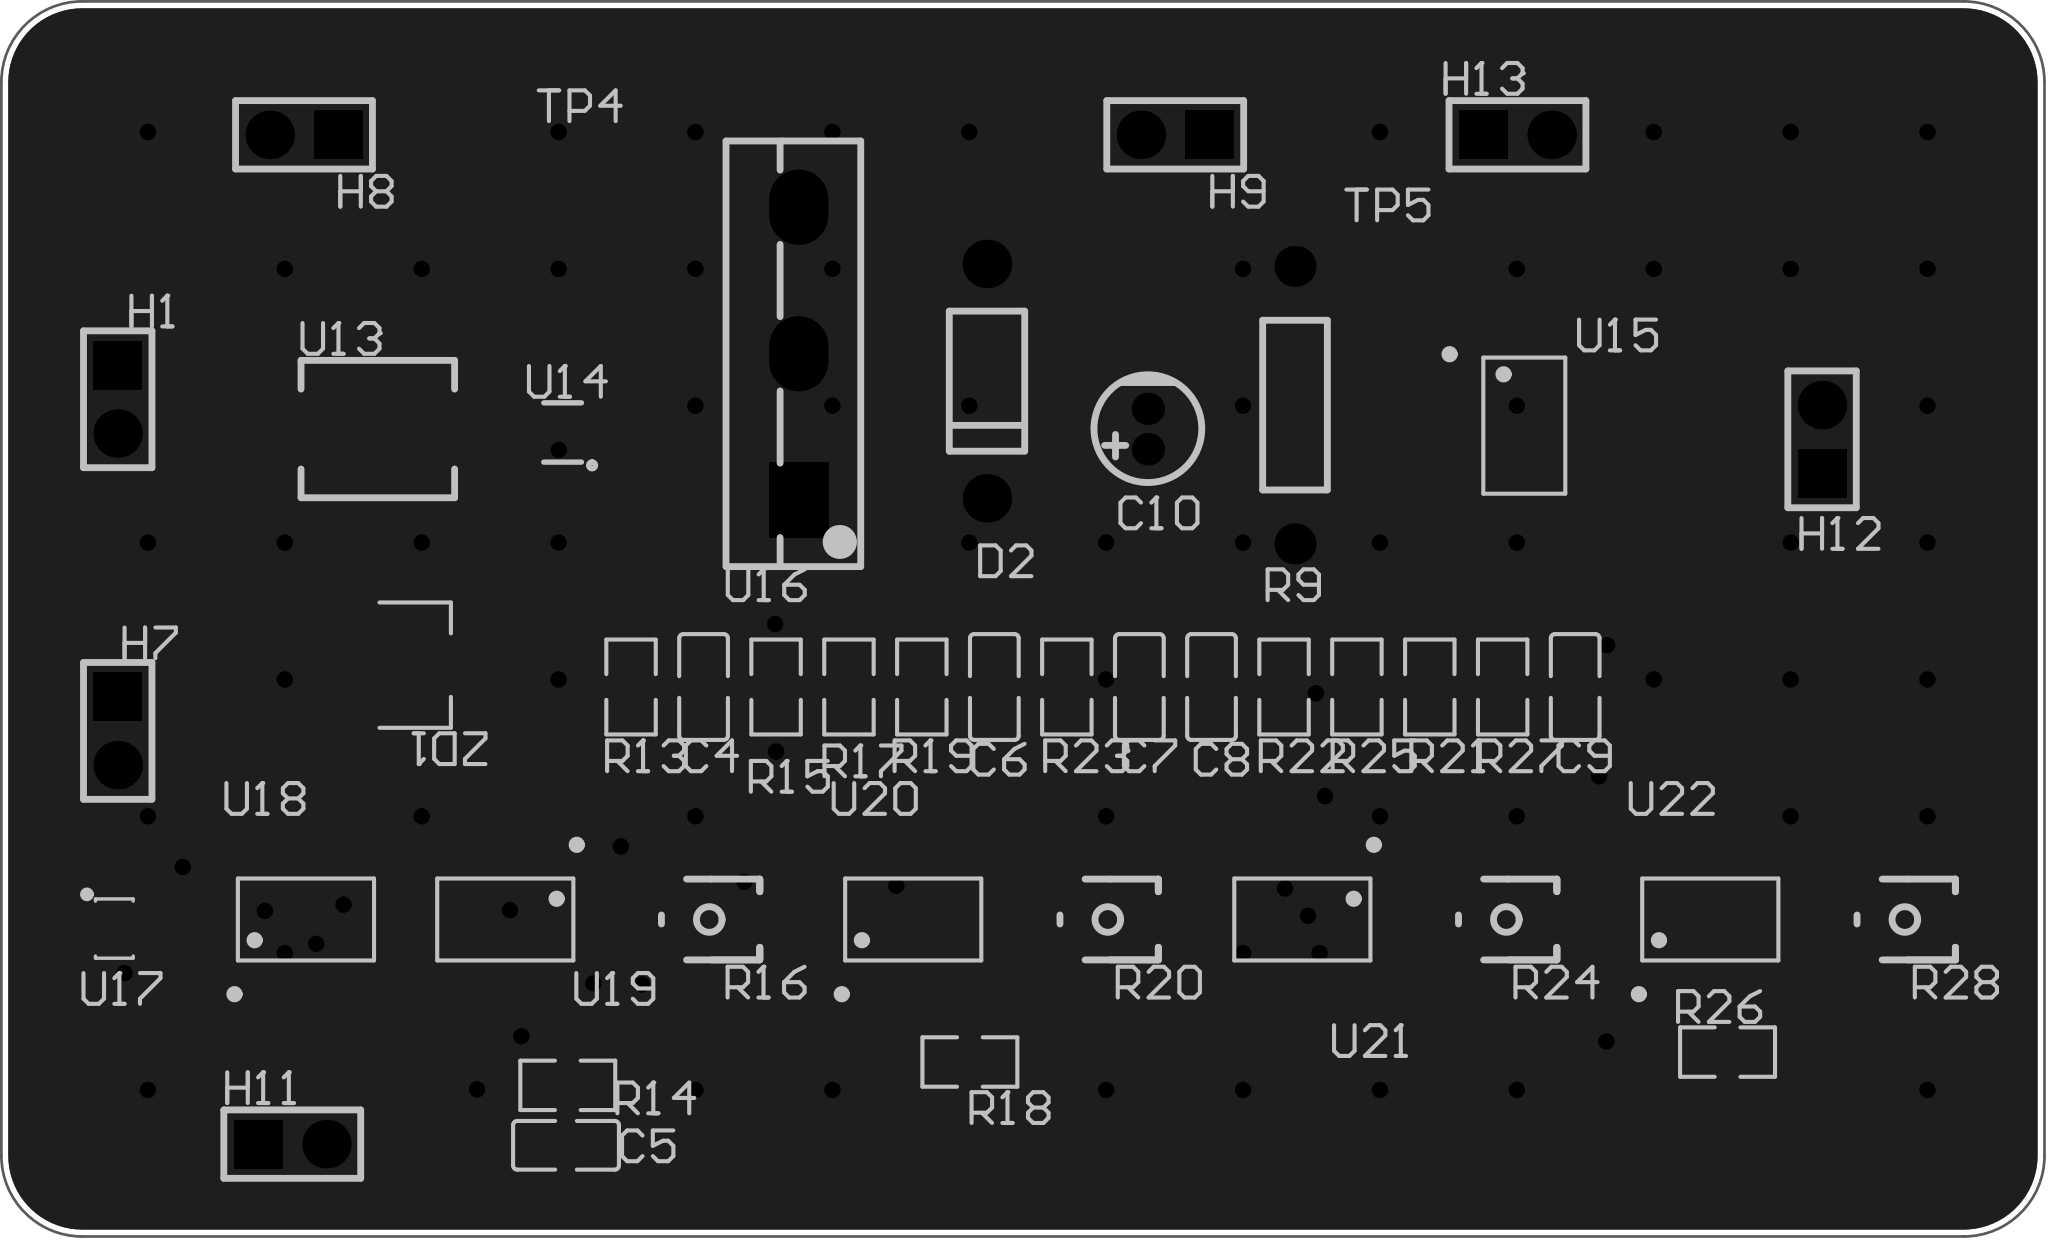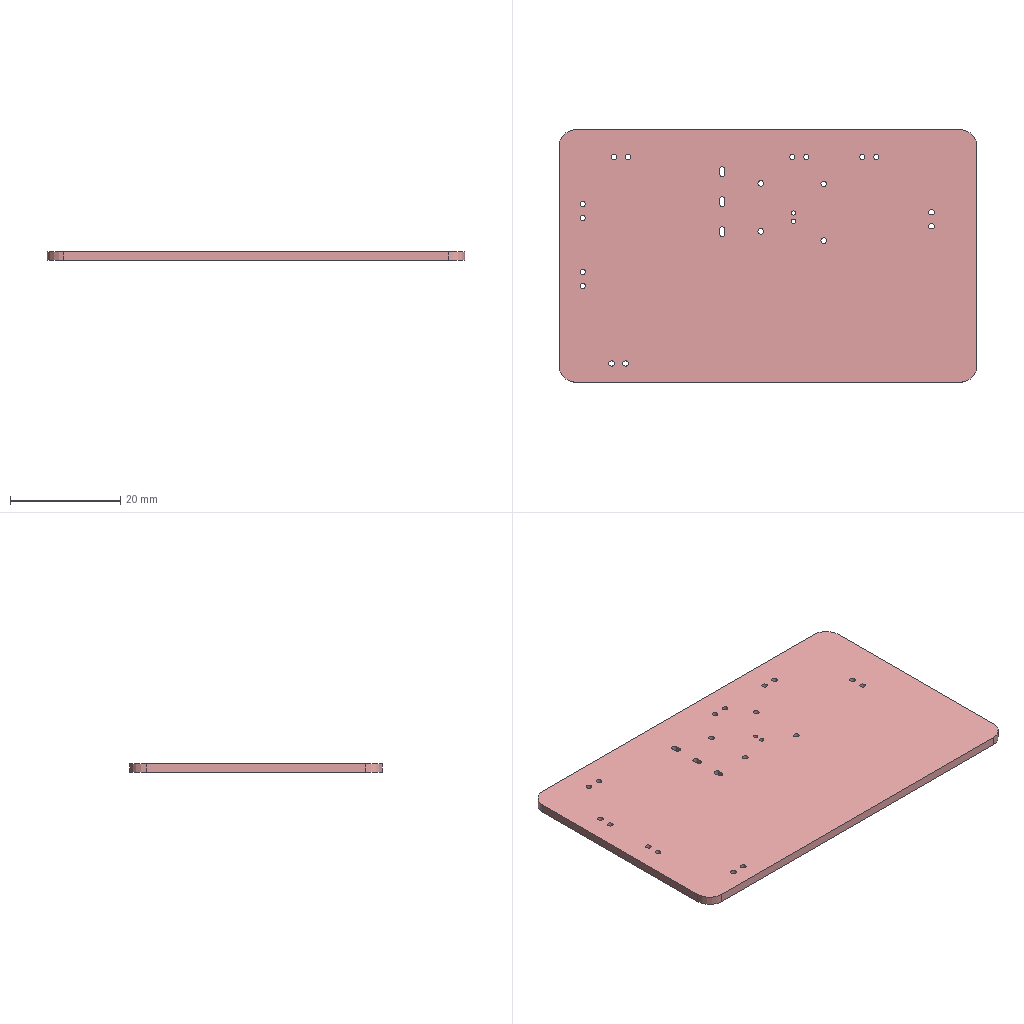Circuit board layout | Altium Designer | box 75.8 x 45.8 x 1.6 mm
Layer stack:
# Altium Designer layer stack of  (unit mm; dielectric type: 0 none, 1 core, 2 prepreg, 3 surface material)
index,name,kind,layer,copper_thickness_mm,dielectric_type,dielectric_thickness_mm,dielectric_material,dielectric_constant
0,Top Paste Mask Layer,other,,,,,,
1,Top Silkscreen Layer,other,,,,,,
2,Top Solder Mask Layer,dielectric,,,3,0.01,,3.3
3,Top Layer,copper,Top Layer,0.035,,,,
4,Dielectric1,dielectric,,,3,1.51,FR4,4.5
5,Bottom Layer,copper,Bottom Layer,0.035,,,,
6,Bottom Solder Mask Layer,dielectric,,,3,0.01,,3.3
7,Bottom Silkscreen Layer,other,,,,,,
8,Bottom Paste Mask Layer,other,,,,,,
# drill layer pairs: low layer,high layer
drill_pair,Top Layer,Bottom Layer
Part placement:
Designator,Comment,Layer,Footprint,Center-X(mm),Center-Y(mm),Rotation
C4,100nF,TopLayer,C0805,105.179,100.407,270
C5,1nF,TopLayer,C0805,100.075,83.395,180
C6,100nF,TopLayer,C0805,115.969,100.407,90
C7,100nF,TopLayer,C0805,121.351,100.407,90
C8,1nF,TopLayer,C0805,124.029,100.407,270
C9,100nF,TopLayer,C0805,137.524,100.407,270
C10,10uF,TopLayer,CAP-TH_BD4.0-P1.50-D0.8-FD,121.666,109.982,90
D2,,TopLayer,DO_1N4007,115.697,111.76,90
H1,,TopLayer,HDR-TH_2P-P2.54-V-M-1,83.439,111.088,270
H7,,TopLayer,HDR-TH_2P-P2.54-V-M-1,83.439,98.777,270
H8,,TopLayer,HDR-TH_2P-P2.54-V-M-1,90.351,120.904,180
H9,,TopLayer,HDR-TH_2P-P2.54-V-M-1,122.682,120.904,180
H11,,TopLayer,HDR-TH_2P-P2.54-V-M-1,89.916,83.439,0
H12,,TopLayer,HDR-TH_2P-P2.54-V-M-1,146.685,109.601,90
H13,,TopLayer,HDR-TH_2P-P2.54-V-M-1,135.382,120.904,0
R9,40,TopLayer,Res_1/4W,127.127,110.871,90
R13,10kΩ,TopLayer,R0805,102.488,100.407,270
R14,10kΩ,TopLayer,R0805,100.14,85.62,180
R15,100Ω,TopLayer,R0805,107.87,100.407,90
R16,100kΩ,TopLayer,RES-ADJ-SMD_VG039NCH,105.366,91.777,180
R17,10kΩ,TopLayer,R0805,110.574,100.407,90
R18,10kΩ,TopLayer,R0805,115.062,86.487,180
R19,1MΩ,TopLayer,R0805,113.278,100.407,90
R20,100kΩ,TopLayer,RES-ADJ-SMD_VG039NCH,120.155,91.777,180
R21,10kΩ,TopLayer,R0805,129.424,100.407,270
R22,10kΩ,TopLayer,R0805,126.72,100.407,270
R23,100Ω,TopLayer,R0805,118.66,100.407,270
R24,100kΩ,TopLayer,RES-ADJ-SMD_VG039NCH,134.944,91.777,180
R25,10kΩ,TopLayer,R0805,132.129,100.407,90
R26,10kΩ,TopLayer,R0805,143.179,86.855,0
R27,1MΩ,TopLayer,R0805,134.833,100.407,270
R28,100kΩ,TopLayer,RES-ADJ-SMD_VG039NCH,149.733,91.777,180
TP4,,TopLayer,Test-Point-0.5mm,98.34,120.347,0
TP5,,TopLayer,Test-Point-0.5mm,130.2,119.458,0
U13,Power inductor (SMD), CKST0502-10uH/M, 10uH, ±20%, 3A, package 5.7mm*5.1mm*2.0mm, Cenke, RoHS,TopLayer,IND-SMD_L5.7-W5.1,93.091,109.982,0
U14,INA199A3DCKT,TopLayer,SC-70-6_L2.1-W1.3-P0.65-LS2.1-BR,99.949,109.855,0
U15,NE5532DR,TopLayer,SOIC-8_L4.9-W3.9-P1.27-LS6.0-BL,135.636,110.109,270
U16,HY5204,TopLayer,TO-247-3_L15.8-W5.0-P5.44-L-1,108.712,112.776,90
U17,SN74LVC2G04DCKR,TopLayer,SOT-363_L2.0-W1.3-P0.65-LS2.1-BR,83.312,91.44,180
U18,NE5532DR,TopLayer,SOIC-8_L4.9-W3.9-P1.27-LS6.0-BL,90.424,91.777,0
U19,UA741CDT,TopLayer,SOIC-8_L4.9-W3.9-P1.27-LS6.0-BL,97.821,91.777,180
U20,UA741CDT,TopLayer,SOIC-8_L4.9-W3.9-P1.27-LS6.0-BL,112.96,91.777,0
U21,UA741CDT,TopLayer,SOIC-8_L4.9-W3.9-P1.27-LS6.0-BL,127.4,91.777,180
U22,UA741CDT,TopLayer,SOIC-8_L4.9-W3.9-P1.27-LS6.0-BL,142.538,91.777,0
ZD1,,TopLayer,SOT-89-3_L4.5-W2.5-P1.50-LS4.2-BR,93.658,101.219,180
Pad and via stacks:
# Altium Designer via and pad stacks of  (unit mm). Each distinct definition once, with the count of objects using it.
# via: kind,start_layer,end_layer,hole_mm,diameter_mm,mode(0 simple;1 top-mid-bottom;2 full stack),diameter_per_layer,count,example_net
# pad: kind,layer,hole_mm,hole_type(0 round;1 square;2 slot),plating,top_size,top_shape(1 round;2 rect;3 octagon;9 rounded rect),mid_size,bottom_size,mode,footprint,size_per_layer,count,example
pad,Top Layer,0,0,plated,1.41x1.35,2,1.41x1.35,1.41x1.35,0,C0805,,12,C4.2
pad,Top Layer,0,0,plated,1.133x1.377,2,1.133x1.377,1.133x1.377,0,R0805,,24,R13.2
pad,Top Layer,0,0,plated,1.6x1.6,2,1.6x1.6,1.6x1.6,0,RES-ADJ-SMD_VG039NCH,,4,R16.2
pad,Top Layer,0,0,plated,1.2x1.5,2,1.2x1.5,1.2x1.5,0,RES-ADJ-SMD_VG039NCH,,8,R16.3
pad,Top Layer,0,0,plated,0.5x0.5,1,0.5x0.5,0.5x0.5,0,Test-Point-0.5mm,,2,TP4.1
pad,Top Layer,0,0,plated,2x2.5,2,2x2.5,2x2.5,0,IND-SMD_L5.7-W5.1,,2,U13.1
pad,Top Layer,0,0,plated,0.42x0.6,2,0.42x0.6,0.42x0.6,0,SC-70-6_L2.1-W1.3-P0.65-LS2.1-BR,,6,U14.1
pad,Top Layer,0,0,plated,0.588x2.045,1,0.588x2.045,0.588x2.045,0,SOIC-8_L4.9-W3.9-P1.27-LS6.0-BL,,48,U15.1
pad,Top Layer,0,0,plated,0.4x0.9,2,0.4x0.9,0.4x0.9,0,SOT-363_L2.0-W1.3-P0.65-LS2.1-BR,,6,U17.2
pad,Top Layer,0,0,plated,1.575x0.672,2,1.575x0.672,1.575x0.672,0,SOT-89-3_L4.5-W2.5-P1.50-LS4.2-BR,,2,ZD1.1
pad,Top Layer,0,0,plated,0.95x0.95,1,0.95x0.95,0.95x0.95,0,SOT-89-3_L4.5-W2.5-P1.50-LS4.2-BR,,1,ZD1.2
pad,Multi-Layer,0.8,0,plated,1.2x1.2,1,1.2x1.2,1.2x1.2,0,CAP-TH_BD4.0-P1.50-D0.8-FD,,2,C10.2
pad,Multi-Layer,1,0,plated,1.8x1.8,1,1.8x1.8,1.8x1.8,0,DO_1N4007,,2,D2.1
pad,Multi-Layer,1,0,plated,1.8x1.8,1,1.8x1.8,1.8x1.8,0,HDR-TH_2P-P2.54-V-M-1,,7,H1.2
pad,Multi-Layer,1,0,plated,1.8x1.8,2,1.8x1.8,1.8x1.8,0,HDR-TH_2P-P2.54-V-M-1,,7,H1.1
pad,Multi-Layer,1,0,plated,1.524x1.524,1,1.524x1.524,1.524x1.524,0,Res_1/4W,,2,R9.1
pad,Multi-Layer,1,2,plated,2.8x2.2,1,2.8x2.2,2.8x2.2,0,TO-247-3_L15.8-W5.0-P5.44-L-1,,2,U16.3
pad,Multi-Layer,1,2,plated,2.8x2.2,2,2.8x2.2,2.8x2.2,0,TO-247-3_L15.8-W5.0-P5.44-L-1,,1,U16.1
via,Top Layer,Bottom Layer,0.3048,0.61,0,,84,$1N5681
Copper pours:
name,layer,net,type(0 solid;1 hatched;2 none)
Top Layer-GND,Top Layer,GND,0
Bottom Layer-GND,Bottom Layer,GND,0
Design rules, without the lines most boards share:
# Altium Designer design rules of  (exported by Altium Designer, unit mm)
# columns: name | kind | enabled | priority | scope1 | scope2 | descriptor | typed fields (field=value)
copperThickness1oz_2 | 2 | enabled | 2 | All | All | Width Constraint (Min=5mil) (Max=100mil) (Preferred=30mil) (All) |
viaSize | 11 | enabled | 1 | All | All | Routing Via (MinHoleWidth=11.811mil) (MaxHoleWidth=248.032mil) (PreferredHoleWidth=12.008mil) (MinWidth=19.685mil) (MaxWidth=393.701mil) (PreferedWidth=24.016mil) (All) | via_min_hole=0.3 via_max_hole=6.3 via_preferred_diameter=0.61 via_preferred_hole=0.305
solderMaskExpansion | 13 | enabled | 2 | All | All | Solder Mask Expansion (Expansion =2.008mil) (All) | expansion=0.051